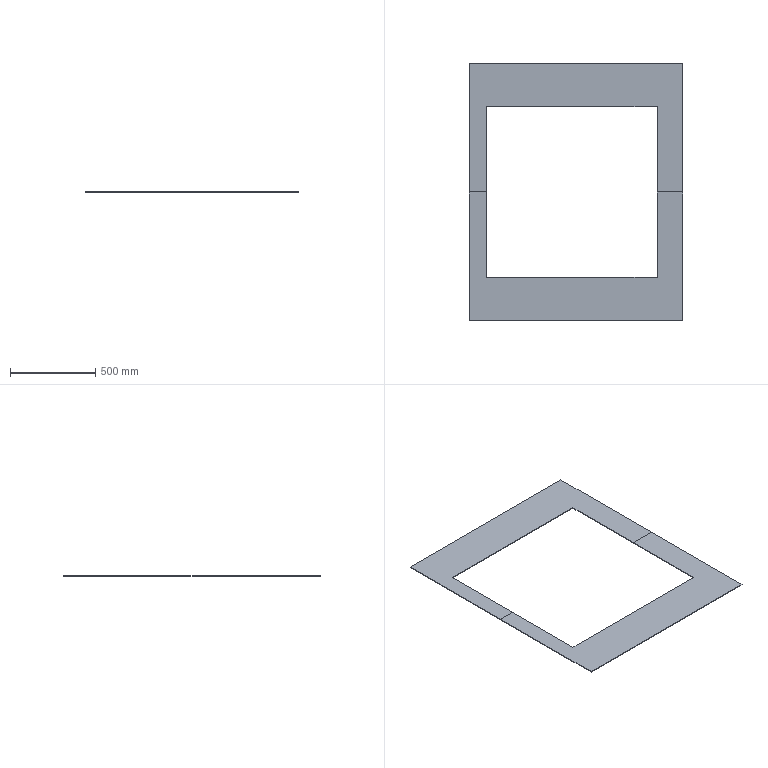Part | STEP file | 电柜通道花纹Plate 2 | 2 solids | 20 faces | box 1250 x 1500 x 4 mm | volume 3500000 mm3 | plane 20
STEP:
#1=CARTESIAN_POINT('',(0.,0.,0.));
#2=DIRECTION('',(0.,0.,1.));
#3=DIRECTION('',(1.,0.,0.));
#4=AXIS2_PLACEMENT_3D('',#1,#2,#3);
#5=CARTESIAN_POINT('',(-128.268,0.,4.));
#6=VERTEX_POINT('',#5);
#7=CARTESIAN_POINT('',(-128.268,0.,0.));
#8=VERTEX_POINT('',#7);
#9=CARTESIAN_POINT('',(-128.268,0.,0.));
#10=DIRECTION('',(0.,0.,-1.));
#11=VECTOR('',#10,1.);
#12=LINE('',#9,#11);
#13=CARTESIAN_POINT('',(-1228.268,0.,-0.01));
#14=DIRECTION('',(0.,-1.,0.));
#15=DIRECTION('',(1.,0.,0.));
#16=AXIS2_PLACEMENT_3D('',#13,#14,#15);
#17=PLANE('',#16);
#18=CARTESIAN_POINT('',(1100.,0.01));
#19=DIRECTION('',(0.,-1.));
#20=VECTOR('',#19,1.);
#21=LINE('',#18,#20);
#22=(GEOMETRIC_REPRESENTATION_CONTEXT(2)PARAMETRIC_REPRESENTATION_CONTEXT()REPRESENTATION_CONTEXT('',''));
#23=DEFINITIONAL_REPRESENTATION('',(#21),#22);
#24=PCURVE('',#17,#23);
#25=CARTESIAN_POINT('',(-128.268,-500.,0.));
#26=DIRECTION('',(1.,0.,0.));
#27=DIRECTION('',(0.,0.,-1.));
#28=AXIS2_PLACEMENT_3D('',#25,#26,#27);
#29=PLANE('',#28);
#30=CARTESIAN_POINT('',(0.,500.));
#31=DIRECTION('',(1.,0.));
#32=VECTOR('',#31,1.);
#33=LINE('',#30,#32);
#34=(GEOMETRIC_REPRESENTATION_CONTEXT(2)PARAMETRIC_REPRESENTATION_CONTEXT()REPRESENTATION_CONTEXT('',''));
#35=DEFINITIONAL_REPRESENTATION('',(#33),#34);
#36=PCURVE('',#29,#35);
#37=SURFACE_CURVE('',#12,(#24,#36),.PCURVE_S1.);
#38=EDGE_CURVE('',#6,#8,#37,.T.);
#39=ORIENTED_EDGE('',*,*,#38,.F.);
#40=CARTESIAN_POINT('',(21.732,0.,4.));
#41=VERTEX_POINT('',#40);
#42=CARTESIAN_POINT('',(0.,0.,4.));
#43=DIRECTION('',(1.,0.,0.));
#44=VECTOR('',#43,1.);
#45=LINE('',#42,#44);
#46=CARTESIAN_POINT('',(1228.268,4.01));
#47=DIRECTION('',(1.,0.));
#48=VECTOR('',#47,1.);
#49=LINE('',#46,#48);
#50=(GEOMETRIC_REPRESENTATION_CONTEXT(2)PARAMETRIC_REPRESENTATION_CONTEXT()REPRESENTATION_CONTEXT('',''));
#51=DEFINITIONAL_REPRESENTATION('',(#49),#50);
#52=PCURVE('',#17,#51);
#53=CARTESIAN_POINT('',(0.,0.,4.));
#54=DIRECTION('',(0.,0.,1.));
#55=DIRECTION('',(1.,0.,0.));
#56=AXIS2_PLACEMENT_3D('',#53,#54,#55);
#57=PLANE('',#56);
#58=CARTESIAN_POINT('',(0.,0.));
#59=DIRECTION('',(1.,0.));
#60=VECTOR('',#59,1.);
#61=LINE('',#58,#60);
#62=(GEOMETRIC_REPRESENTATION_CONTEXT(2)PARAMETRIC_REPRESENTATION_CONTEXT()REPRESENTATION_CONTEXT('',''));
#63=DEFINITIONAL_REPRESENTATION('',(#61),#62);
#64=PCURVE('',#57,#63);
#65=SURFACE_CURVE('',#45,(#52,#64),.PCURVE_S1.);
#66=EDGE_CURVE('',#6,#41,#65,.T.);
#67=ORIENTED_EDGE('',*,*,#66,.T.);
#68=CARTESIAN_POINT('',(21.732,0.,0.));
#69=VERTEX_POINT('',#68);
#70=CARTESIAN_POINT('',(21.732,0.,4.));
#71=DIRECTION('',(0.,0.,1.));
#72=VECTOR('',#71,1.);
#73=LINE('',#70,#72);
#74=CARTESIAN_POINT('',(1250.,4.01));
#75=DIRECTION('',(0.,1.));
#76=VECTOR('',#75,1.);
#77=LINE('',#74,#76);
#78=(GEOMETRIC_REPRESENTATION_CONTEXT(2)PARAMETRIC_REPRESENTATION_CONTEXT()REPRESENTATION_CONTEXT('',''));
#79=DEFINITIONAL_REPRESENTATION('',(#77),#78);
#80=PCURVE('',#17,#79);
#81=CARTESIAN_POINT('',(21.732,750.,4.));
#82=DIRECTION('',(-1.,0.,0.));
#83=DIRECTION('',(0.,-1.,0.));
#84=AXIS2_PLACEMENT_3D('',#81,#82,#83);
#85=PLANE('',#84);
#86=CARTESIAN_POINT('',(750.,0.));
#87=DIRECTION('',(0.,1.));
#88=VECTOR('',#87,1.);
#89=LINE('',#86,#88);
#90=(GEOMETRIC_REPRESENTATION_CONTEXT(2)PARAMETRIC_REPRESENTATION_CONTEXT()REPRESENTATION_CONTEXT('',''));
#91=DEFINITIONAL_REPRESENTATION('',(#89),#90);
#92=PCURVE('',#85,#91);
#93=SURFACE_CURVE('',#73,(#80,#92),.PCURVE_S1.);
#94=EDGE_CURVE('',#69,#41,#93,.T.);
#95=ORIENTED_EDGE('',*,*,#94,.F.);
#96=CARTESIAN_POINT('',(0.,0.,0.));
#97=DIRECTION('',(1.,0.,0.));
#98=VECTOR('',#97,1.);
#99=LINE('',#96,#98);
#100=CARTESIAN_POINT('',(1228.268,0.01));
#101=DIRECTION('',(1.,0.));
#102=VECTOR('',#101,1.);
#103=LINE('',#100,#102);
#104=(GEOMETRIC_REPRESENTATION_CONTEXT(2)PARAMETRIC_REPRESENTATION_CONTEXT()REPRESENTATION_CONTEXT('',''));
#105=DEFINITIONAL_REPRESENTATION('',(#103),#104);
#106=PCURVE('',#17,#105);
#107=CARTESIAN_POINT('',(0.,0.,0.));
#108=DIRECTION('',(0.,0.,1.));
#109=DIRECTION('',(1.,0.,0.));
#110=AXIS2_PLACEMENT_3D('',#107,#108,#109);
#111=PLANE('',#110);
#112=CARTESIAN_POINT('',(0.,0.));
#113=DIRECTION('',(1.,0.));
#114=VECTOR('',#113,1.);
#115=LINE('',#112,#114);
#116=(GEOMETRIC_REPRESENTATION_CONTEXT(2)PARAMETRIC_REPRESENTATION_CONTEXT()REPRESENTATION_CONTEXT('',''));
#117=DEFINITIONAL_REPRESENTATION('',(#115),#116);
#118=PCURVE('',#111,#117);
#119=SURFACE_CURVE('',#99,(#106,#118),.PCURVE_S1.);
#120=EDGE_CURVE('',#8,#69,#119,.T.);
#121=ORIENTED_EDGE('',*,*,#120,.F.);
#122=EDGE_LOOP('',(#39,#67,#95,#121));
#123=FACE_BOUND('',#122,.T.);
#124=ADVANCED_FACE('',(#123),#17,.F.);
#125=CARTESIAN_POINT('',(-1228.268,0.,4.));
#126=VERTEX_POINT('',#125);
#127=CARTESIAN_POINT('',(-1228.268,0.,0.));
#128=VERTEX_POINT('',#127);
#129=CARTESIAN_POINT('',(-1228.268,0.,4.));
#130=DIRECTION('',(0.,0.,-1.));
#131=VECTOR('',#130,1.);
#132=LINE('',#129,#131);
#133=CARTESIAN_POINT('',(-1228.268,0.,-0.01));
#134=DIRECTION('',(0.,-1.,0.));
#135=DIRECTION('',(1.,0.,0.));
#136=AXIS2_PLACEMENT_3D('',#133,#134,#135);
#137=PLANE('',#136);
#138=CARTESIAN_POINT('',(0.,4.01));
#139=DIRECTION('',(0.,-1.));
#140=VECTOR('',#139,1.);
#141=LINE('',#138,#140);
#142=(GEOMETRIC_REPRESENTATION_CONTEXT(2)PARAMETRIC_REPRESENTATION_CONTEXT()REPRESENTATION_CONTEXT('',''));
#143=DEFINITIONAL_REPRESENTATION('',(#141),#142);
#144=PCURVE('',#137,#143);
#145=CARTESIAN_POINT('',(-1228.268,750.,4.));
#146=DIRECTION('',(1.,0.,0.));
#147=DIRECTION('',(0.,1.,0.));
#148=AXIS2_PLACEMENT_3D('',#145,#146,#147);
#149=PLANE('',#148);
#150=CARTESIAN_POINT('',(-750.,0.));
#151=DIRECTION('',(0.,-1.));
#152=VECTOR('',#151,1.);
#153=LINE('',#150,#152);
#154=(GEOMETRIC_REPRESENTATION_CONTEXT(2)PARAMETRIC_REPRESENTATION_CONTEXT()REPRESENTATION_CONTEXT('',''));
#155=DEFINITIONAL_REPRESENTATION('',(#153),#154);
#156=PCURVE('',#149,#155);
#157=SURFACE_CURVE('',#132,(#144,#156),.PCURVE_S1.);
#158=EDGE_CURVE('',#126,#128,#157,.T.);
#159=ORIENTED_EDGE('',*,*,#158,.F.);
#160=CARTESIAN_POINT('',(-1128.268,0.,4.));
#161=VERTEX_POINT('',#160);
#162=CARTESIAN_POINT('',(0.,0.,4.));
#163=DIRECTION('',(1.,0.,0.));
#164=VECTOR('',#163,1.);
#165=LINE('',#162,#164);
#166=CARTESIAN_POINT('',(1228.268,4.01));
#167=DIRECTION('',(1.,0.));
#168=VECTOR('',#167,1.);
#169=LINE('',#166,#168);
#170=(GEOMETRIC_REPRESENTATION_CONTEXT(2)PARAMETRIC_REPRESENTATION_CONTEXT()REPRESENTATION_CONTEXT('',''));
#171=DEFINITIONAL_REPRESENTATION('',(#169),#170);
#172=PCURVE('',#137,#171);
#173=CARTESIAN_POINT('',(0.,0.));
#174=DIRECTION('',(1.,0.));
#175=VECTOR('',#174,1.);
#176=LINE('',#173,#175);
#177=(GEOMETRIC_REPRESENTATION_CONTEXT(2)PARAMETRIC_REPRESENTATION_CONTEXT()REPRESENTATION_CONTEXT('',''));
#178=DEFINITIONAL_REPRESENTATION('',(#176),#177);
#179=PCURVE('',#57,#178);
#180=SURFACE_CURVE('',#165,(#172,#179),.PCURVE_S1.);
#181=EDGE_CURVE('',#126,#161,#180,.T.);
#182=ORIENTED_EDGE('',*,*,#181,.T.);
#183=CARTESIAN_POINT('',(-1128.268,0.,0.));
#184=VERTEX_POINT('',#183);
#185=CARTESIAN_POINT('',(-1128.268,0.,0.));
#186=DIRECTION('',(0.,0.,1.));
#187=VECTOR('',#186,1.);
#188=LINE('',#185,#187);
#189=CARTESIAN_POINT('',(100.,0.01));
#190=DIRECTION('',(0.,1.));
#191=VECTOR('',#190,1.);
#192=LINE('',#189,#191);
#193=(GEOMETRIC_REPRESENTATION_CONTEXT(2)PARAMETRIC_REPRESENTATION_CONTEXT()REPRESENTATION_CONTEXT('',''));
#194=DEFINITIONAL_REPRESENTATION('',(#192),#193);
#195=PCURVE('',#137,#194);
#196=CARTESIAN_POINT('',(-1128.268,-500.,0.));
#197=DIRECTION('',(-1.,0.,0.));
#198=DIRECTION('',(0.,0.,1.));
#199=AXIS2_PLACEMENT_3D('',#196,#197,#198);
#200=PLANE('',#199);
#201=CARTESIAN_POINT('',(0.,500.));
#202=DIRECTION('',(1.,0.));
#203=VECTOR('',#202,1.);
#204=LINE('',#201,#203);
#205=(GEOMETRIC_REPRESENTATION_CONTEXT(2)PARAMETRIC_REPRESENTATION_CONTEXT()REPRESENTATION_CONTEXT('',''));
#206=DEFINITIONAL_REPRESENTATION('',(#204),#205);
#207=PCURVE('',#200,#206);
#208=SURFACE_CURVE('',#188,(#195,#207),.PCURVE_S1.);
#209=EDGE_CURVE('',#184,#161,#208,.T.);
#210=ORIENTED_EDGE('',*,*,#209,.F.);
#211=CARTESIAN_POINT('',(0.,0.,0.));
#212=DIRECTION('',(1.,0.,0.));
#213=VECTOR('',#212,1.);
#214=LINE('',#211,#213);
#215=CARTESIAN_POINT('',(1228.268,0.01));
#216=DIRECTION('',(1.,0.));
#217=VECTOR('',#216,1.);
#218=LINE('',#215,#217);
#219=(GEOMETRIC_REPRESENTATION_CONTEXT(2)PARAMETRIC_REPRESENTATION_CONTEXT()REPRESENTATION_CONTEXT('',''));
#220=DEFINITIONAL_REPRESENTATION('',(#218),#219);
#221=PCURVE('',#137,#220);
#222=CARTESIAN_POINT('',(0.,0.));
#223=DIRECTION('',(1.,0.));
#224=VECTOR('',#223,1.);
#225=LINE('',#222,#224);
#226=(GEOMETRIC_REPRESENTATION_CONTEXT(2)PARAMETRIC_REPRESENTATION_CONTEXT()REPRESENTATION_CONTEXT('',''));
#227=DEFINITIONAL_REPRESENTATION('',(#225),#226);
#228=PCURVE('',#111,#227);
#229=SURFACE_CURVE('',#214,(#221,#228),.PCURVE_S1.);
#230=EDGE_CURVE('',#128,#184,#229,.T.);
#231=ORIENTED_EDGE('',*,*,#230,.F.);
#232=EDGE_LOOP('',(#159,#182,#210,#231));
#233=FACE_BOUND('',#232,.T.);
#234=ADVANCED_FACE('',(#233),#137,.F.);
#235=CARTESIAN_POINT('',(-128.268,-500.,4.));
#236=VERTEX_POINT('',#235);
#237=CARTESIAN_POINT('',(-128.268,-500.,4.));
#238=DIRECTION('',(0.,1.,0.));
#239=VECTOR('',#238,1.);
#240=LINE('',#237,#239);
#241=CARTESIAN_POINT('',(-4.,0.));
#242=DIRECTION('',(0.,1.));
#243=VECTOR('',#242,1.);
#244=LINE('',#241,#243);
#245=(GEOMETRIC_REPRESENTATION_CONTEXT(2)PARAMETRIC_REPRESENTATION_CONTEXT()REPRESENTATION_CONTEXT('',''));
#246=DEFINITIONAL_REPRESENTATION('',(#244),#245);
#247=PCURVE('',#29,#246);
#248=CARTESIAN_POINT('',(-128.268,-500.));
#249=DIRECTION('',(0.,1.));
#250=VECTOR('',#249,1.);
#251=LINE('',#248,#250);
#252=(GEOMETRIC_REPRESENTATION_CONTEXT(2)PARAMETRIC_REPRESENTATION_CONTEXT()REPRESENTATION_CONTEXT('',''));
#253=DEFINITIONAL_REPRESENTATION('',(#251),#252);
#254=PCURVE('',#57,#253);
#255=SURFACE_CURVE('',#240,(#247,#254),.PCURVE_S1.);
#256=EDGE_CURVE('',#236,#6,#255,.T.);
#257=ORIENTED_EDGE('',*,*,#256,.T.);
#258=ORIENTED_EDGE('',*,*,#38,.T.);
#259=CARTESIAN_POINT('',(-128.268,-500.,0.));
#260=VERTEX_POINT('',#259);
#261=CARTESIAN_POINT('',(-128.268,-500.,0.));
#262=DIRECTION('',(0.,1.,0.));
#263=VECTOR('',#262,1.);
#264=LINE('',#261,#263);
#265=CARTESIAN_POINT('',(0.,0.));
#266=DIRECTION('',(0.,1.));
#267=VECTOR('',#266,1.);
#268=LINE('',#265,#267);
#269=(GEOMETRIC_REPRESENTATION_CONTEXT(2)PARAMETRIC_REPRESENTATION_CONTEXT()REPRESENTATION_CONTEXT('',''));
#270=DEFINITIONAL_REPRESENTATION('',(#268),#269);
#271=PCURVE('',#29,#270);
#272=CARTESIAN_POINT('',(-128.268,-500.));
#273=DIRECTION('',(0.,1.));
#274=VECTOR('',#273,1.);
#275=LINE('',#272,#274);
#276=(GEOMETRIC_REPRESENTATION_CONTEXT(2)PARAMETRIC_REPRESENTATION_CONTEXT()REPRESENTATION_CONTEXT('',''));
#277=DEFINITIONAL_REPRESENTATION('',(#275),#276);
#278=PCURVE('',#111,#277);
#279=SURFACE_CURVE('',#264,(#271,#278),.PCURVE_S1.);
#280=EDGE_CURVE('',#260,#8,#279,.T.);
#281=ORIENTED_EDGE('',*,*,#280,.F.);
#282=CARTESIAN_POINT('',(-128.268,-500.,0.));
#283=DIRECTION('',(0.,0.,1.));
#284=VECTOR('',#283,1.);
#285=LINE('',#282,#284);
#286=CARTESIAN_POINT('',(0.,0.));
#287=DIRECTION('',(-1.,0.));
#288=VECTOR('',#287,1.);
#289=LINE('',#286,#288);
#290=(GEOMETRIC_REPRESENTATION_CONTEXT(2)PARAMETRIC_REPRESENTATION_CONTEXT()REPRESENTATION_CONTEXT('',''));
#291=DEFINITIONAL_REPRESENTATION('',(#289),#290);
#292=PCURVE('',#29,#291);
#293=CARTESIAN_POINT('',(-1128.268,-500.,0.));
#294=DIRECTION('',(0.,-1.,0.));
#295=DIRECTION('',(0.,0.,-1.));
#296=AXIS2_PLACEMENT_3D('',#293,#294,#295);
#297=PLANE('',#296);
#298=CARTESIAN_POINT('',(0.,1000.));
#299=DIRECTION('',(-1.,0.));
#300=VECTOR('',#299,1.);
#301=LINE('',#298,#300);
#302=(GEOMETRIC_REPRESENTATION_CONTEXT(2)PARAMETRIC_REPRESENTATION_CONTEXT()REPRESENTATION_CONTEXT('',''));
#303=DEFINITIONAL_REPRESENTATION('',(#301),#302);
#304=PCURVE('',#297,#303);
#305=SURFACE_CURVE('',#285,(#292,#304),.PCURVE_S1.);
#306=EDGE_CURVE('',#260,#236,#305,.T.);
#307=ORIENTED_EDGE('',*,*,#306,.T.);
#308=EDGE_LOOP('',(#257,#258,#281,#307));
#309=FACE_BOUND('',#308,.T.);
#310=ADVANCED_FACE('',(#309),#29,.F.);
#311=CARTESIAN_POINT('',(-1128.268,-500.,0.));
#312=VERTEX_POINT('',#311);
#313=CARTESIAN_POINT('',(-1128.268,-500.,0.));
#314=DIRECTION('',(0.,-1.,0.));
#315=VECTOR('',#314,1.);
#316=LINE('',#313,#315);
#317=CARTESIAN_POINT('',(0.,0.));
#318=DIRECTION('',(0.,-1.));
#319=VECTOR('',#318,1.);
#320=LINE('',#317,#319);
#321=(GEOMETRIC_REPRESENTATION_CONTEXT(2)PARAMETRIC_REPRESENTATION_CONTEXT()REPRESENTATION_CONTEXT('',''));
#322=DEFINITIONAL_REPRESENTATION('',(#320),#321);
#323=PCURVE('',#200,#322);
#324=CARTESIAN_POINT('',(-1128.268,-500.));
#325=DIRECTION('',(0.,-1.));
#326=VECTOR('',#325,1.);
#327=LINE('',#324,#326);
#328=(GEOMETRIC_REPRESENTATION_CONTEXT(2)PARAMETRIC_REPRESENTATION_CONTEXT()REPRESENTATION_CONTEXT('',''));
#329=DEFINITIONAL_REPRESENTATION('',(#327),#328);
#330=PCURVE('',#111,#329);
#331=SURFACE_CURVE('',#316,(#323,#330),.PCURVE_S1.);
#332=EDGE_CURVE('',#184,#312,#331,.T.);
#333=ORIENTED_EDGE('',*,*,#332,.F.);
#334=ORIENTED_EDGE('',*,*,#209,.T.);
#335=CARTESIAN_POINT('',(-1128.268,-500.,4.));
#336=VERTEX_POINT('',#335);
#337=CARTESIAN_POINT('',(-1128.268,-500.,4.));
#338=DIRECTION('',(0.,-1.,0.));
#339=VECTOR('',#338,1.);
#340=LINE('',#337,#339);
#341=CARTESIAN_POINT('',(4.,0.));
#342=DIRECTION('',(0.,-1.));
#343=VECTOR('',#342,1.);
#344=LINE('',#341,#343);
#345=(GEOMETRIC_REPRESENTATION_CONTEXT(2)PARAMETRIC_REPRESENTATION_CONTEXT()REPRESENTATION_CONTEXT('',''));
#346=DEFINITIONAL_REPRESENTATION('',(#344),#345);
#347=PCURVE('',#200,#346);
#348=CARTESIAN_POINT('',(-1128.268,-500.));
#349=DIRECTION('',(0.,-1.));
#350=VECTOR('',#349,1.);
#351=LINE('',#348,#350);
#352=(GEOMETRIC_REPRESENTATION_CONTEXT(2)PARAMETRIC_REPRESENTATION_CONTEXT()REPRESENTATION_CONTEXT('',''));
#353=DEFINITIONAL_REPRESENTATION('',(#351),#352);
#354=PCURVE('',#57,#353);
#355=SURFACE_CURVE('',#340,(#347,#354),.PCURVE_S1.);
#356=EDGE_CURVE('',#161,#336,#355,.T.);
#357=ORIENTED_EDGE('',*,*,#356,.T.);
#358=CARTESIAN_POINT('',(-1128.268,-500.,0.));
#359=DIRECTION('',(0.,0.,1.));
#360=VECTOR('',#359,1.);
#361=LINE('',#358,#360);
#362=CARTESIAN_POINT('',(0.,0.));
#363=DIRECTION('',(1.,0.));
#364=VECTOR('',#363,1.);
#365=LINE('',#362,#364);
#366=(GEOMETRIC_REPRESENTATION_CONTEXT(2)PARAMETRIC_REPRESENTATION_CONTEXT()REPRESENTATION_CONTEXT('',''));
#367=DEFINITIONAL_REPRESENTATION('',(#365),#366);
#368=PCURVE('',#200,#367);
#369=CARTESIAN_POINT('',(0.,0.));
#370=DIRECTION('',(-1.,0.));
#371=VECTOR('',#370,1.);
#372=LINE('',#369,#371);
#373=(GEOMETRIC_REPRESENTATION_CONTEXT(2)PARAMETRIC_REPRESENTATION_CONTEXT()REPRESENTATION_CONTEXT('',''));
#374=DEFINITIONAL_REPRESENTATION('',(#372),#373);
#375=PCURVE('',#297,#374);
#376=SURFACE_CURVE('',#361,(#368,#375),.PCURVE_S1.);
#377=EDGE_CURVE('',#312,#336,#376,.T.);
#378=ORIENTED_EDGE('',*,*,#377,.F.);
#379=EDGE_LOOP('',(#333,#334,#357,#378));
#380=FACE_BOUND('',#379,.T.);
#381=ADVANCED_FACE('',(#380),#200,.F.);
#382=CARTESIAN_POINT('',(-1228.268,-750.,0.));
#383=VERTEX_POINT('',#382);
#384=CARTESIAN_POINT('',(-1228.268,750.,0.));
#385=DIRECTION('',(0.,-1.,0.));
#386=VECTOR('',#385,1.);
#387=LINE('',#384,#386);
#388=CARTESIAN_POINT('',(-1228.268,750.));
#389=DIRECTION('',(0.,-1.));
#390=VECTOR('',#389,1.);
#391=LINE('',#388,#390);
#392=(GEOMETRIC_REPRESENTATION_CONTEXT(2)PARAMETRIC_REPRESENTATION_CONTEXT()REPRESENTATION_CONTEXT('',''));
#393=DEFINITIONAL_REPRESENTATION('',(#391),#392);
#394=PCURVE('',#111,#393);
#395=CARTESIAN_POINT('',(0.,-4.));
#396=DIRECTION('',(-1.,0.));
#397=VECTOR('',#396,1.);
#398=LINE('',#395,#397);
#399=(GEOMETRIC_REPRESENTATION_CONTEXT(2)PARAMETRIC_REPRESENTATION_CONTEXT()REPRESENTATION_CONTEXT('',''));
#400=DEFINITIONAL_REPRESENTATION('',(#398),#399);
#401=PCURVE('',#149,#400);
#402=SURFACE_CURVE('',#387,(#394,#401),.PCURVE_S1.);
#403=EDGE_CURVE('',#128,#383,#402,.T.);
#404=ORIENTED_EDGE('',*,*,#403,.F.);
#405=ORIENTED_EDGE('',*,*,#230,.T.);
#406=ORIENTED_EDGE('',*,*,#332,.T.);
#407=CARTESIAN_POINT('',(-1128.268,-500.,0.));
#408=DIRECTION('',(1.,0.,0.));
#409=VECTOR('',#408,1.);
#410=LINE('',#407,#409);
#411=CARTESIAN_POINT('',(-1128.268,-500.));
#412=DIRECTION('',(1.,0.));
#413=VECTOR('',#412,1.);
#414=LINE('',#411,#413);
#415=(GEOMETRIC_REPRESENTATION_CONTEXT(2)PARAMETRIC_REPRESENTATION_CONTEXT()REPRESENTATION_CONTEXT('',''));
#416=DEFINITIONAL_REPRESENTATION('',(#414),#415);
#417=PCURVE('',#111,#416);
#418=CARTESIAN_POINT('',(0.,0.));
#419=DIRECTION('',(0.,1.));
#420=VECTOR('',#419,1.);
#421=LINE('',#418,#420);
#422=(GEOMETRIC_REPRESENTATION_CONTEXT(2)PARAMETRIC_REPRESENTATION_CONTEXT()REPRESENTATION_CONTEXT('',''));
#423=DEFINITIONAL_REPRESENTATION('',(#421),#422);
#424=PCURVE('',#297,#423);
#425=SURFACE_CURVE('',#410,(#417,#424),.PCURVE_S1.);
#426=EDGE_CURVE('',#312,#260,#425,.T.);
#427=ORIENTED_EDGE('',*,*,#426,.T.);
#428=ORIENTED_EDGE('',*,*,#280,.T.);
#429=ORIENTED_EDGE('',*,*,#120,.T.);
#430=CARTESIAN_POINT('',(21.732,-750.,0.));
#431=VERTEX_POINT('',#430);
#432=CARTESIAN_POINT('',(21.732,750.,0.));
#433=DIRECTION('',(0.,1.,0.));
#434=VECTOR('',#433,1.);
#435=LINE('',#432,#434);
#436=CARTESIAN_POINT('',(21.732,750.));
#437=DIRECTION('',(0.,1.));
#438=VECTOR('',#437,1.);
#439=LINE('',#436,#438);
#440=(GEOMETRIC_REPRESENTATION_CONTEXT(2)PARAMETRIC_REPRESENTATION_CONTEXT()REPRESENTATION_CONTEXT('',''));
#441=DEFINITIONAL_REPRESENTATION('',(#439),#440);
#442=PCURVE('',#111,#441);
#443=CARTESIAN_POINT('',(0.,-4.));
#444=DIRECTION('',(-1.,0.));
#445=VECTOR('',#444,1.);
#446=LINE('',#443,#445);
#447=(GEOMETRIC_REPRESENTATION_CONTEXT(2)PARAMETRIC_REPRESENTATION_CONTEXT()REPRESENTATION_CONTEXT('',''));
#448=DEFINITIONAL_REPRESENTATION('',(#446),#447);
#449=PCURVE('',#85,#448);
#450=SURFACE_CURVE('',#435,(#442,#449),.PCURVE_S1.);
#451=EDGE_CURVE('',#431,#69,#450,.T.);
#452=ORIENTED_EDGE('',*,*,#451,.F.);
#453=CARTESIAN_POINT('',(-1228.268,-750.,0.));
#454=DIRECTION('',(1.,0.,0.));
#455=VECTOR('',#454,1.);
#456=LINE('',#453,#455);
#457=CARTESIAN_POINT('',(-1228.268,-750.));
#458=DIRECTION('',(1.,0.));
#459=VECTOR('',#458,1.);
#460=LINE('',#457,#459);
#461=(GEOMETRIC_REPRESENTATION_CONTEXT(2)PARAMETRIC_REPRESENTATION_CONTEXT()REPRESENTATION_CONTEXT('',''));
#462=DEFINITIONAL_REPRESENTATION('',(#460),#461);
#463=PCURVE('',#111,#462);
#464=CARTESIAN_POINT('',(-1228.268,-750.,4.));
#465=DIRECTION('',(0.,1.,0.));
#466=DIRECTION('',(0.,0.,1.));
#467=AXIS2_PLACEMENT_3D('',#464,#465,#466);
#468=PLANE('',#467);
#469=CARTESIAN_POINT('',(-4.,0.));
#470=DIRECTION('',(0.,1.));
#471=VECTOR('',#470,1.);
#472=LINE('',#469,#471);
#473=(GEOMETRIC_REPRESENTATION_CONTEXT(2)PARAMETRIC_REPRESENTATION_CONTEXT()REPRESENTATION_CONTEXT('',''));
#474=DEFINITIONAL_REPRESENTATION('',(#472),#473);
#475=PCURVE('',#468,#474);
#476=SURFACE_CURVE('',#456,(#463,#475),.PCURVE_S1.);
#477=EDGE_CURVE('',#383,#431,#476,.T.);
#478=ORIENTED_EDGE('',*,*,#477,.F.);
#479=EDGE_LOOP('',(#404,#405,#406,#427,#428,#429,#452,#478));
#480=FACE_BOUND('',#479,.T.);
#481=ADVANCED_FACE('',(#480),#111,.F.);
#482=ORIENTED_EDGE('',*,*,#181,.F.);
#483=CARTESIAN_POINT('',(-1228.268,-750.,4.));
#484=VERTEX_POINT('',#483);
#485=CARTESIAN_POINT('',(-1228.268,750.,4.));
#486=DIRECTION('',(0.,-1.,0.));
#487=VECTOR('',#486,1.);
#488=LINE('',#485,#487);
#489=CARTESIAN_POINT('',(-1228.268,750.));
#490=DIRECTION('',(0.,-1.));
#491=VECTOR('',#490,1.);
#492=LINE('',#489,#491);
#493=(GEOMETRIC_REPRESENTATION_CONTEXT(2)PARAMETRIC_REPRESENTATION_CONTEXT()REPRESENTATION_CONTEXT('',''));
#494=DEFINITIONAL_REPRESENTATION('',(#492),#493);
#495=PCURVE('',#57,#494);
#496=CARTESIAN_POINT('',(0.,0.));
#497=DIRECTION('',(-1.,0.));
#498=VECTOR('',#497,1.);
#499=LINE('',#496,#498);
#500=(GEOMETRIC_REPRESENTATION_CONTEXT(2)PARAMETRIC_REPRESENTATION_CONTEXT()REPRESENTATION_CONTEXT('',''));
#501=DEFINITIONAL_REPRESENTATION('',(#499),#500);
#502=PCURVE('',#149,#501);
#503=SURFACE_CURVE('',#488,(#495,#502),.PCURVE_S1.);
#504=EDGE_CURVE('',#126,#484,#503,.T.);
#505=ORIENTED_EDGE('',*,*,#504,.T.);
#506=CARTESIAN_POINT('',(21.732,-750.,4.));
#507=VERTEX_POINT('',#506);
#508=CARTESIAN_POINT('',(-1228.268,-750.,4.));
#509=DIRECTION('',(1.,0.,0.));
#510=VECTOR('',#509,1.);
#511=LINE('',#508,#510);
#512=CARTESIAN_POINT('',(-1228.268,-750.));
#513=DIRECTION('',(1.,0.));
#514=VECTOR('',#513,1.);
#515=LINE('',#512,#514);
#516=(GEOMETRIC_REPRESENTATION_CONTEXT(2)PARAMETRIC_REPRESENTATION_CONTEXT()REPRESENTATION_CONTEXT('',''));
#517=DEFINITIONAL_REPRESENTATION('',(#515),#516);
#518=PCURVE('',#57,#517);
#519=CARTESIAN_POINT('',(0.,0.));
#520=DIRECTION('',(0.,1.));
#521=VECTOR('',#520,1.);
#522=LINE('',#519,#521);
#523=(GEOMETRIC_REPRESENTATION_CONTEXT(2)PARAMETRIC_REPRESENTATION_CONTEXT()REPRESENTATION_CONTEXT('',''));
#524=DEFINITIONAL_REPRESENTATION('',(#522),#523);
#525=PCURVE('',#468,#524);
#526=SURFACE_CURVE('',#511,(#518,#525),.PCURVE_S1.);
#527=EDGE_CURVE('',#484,#507,#526,.T.);
#528=ORIENTED_EDGE('',*,*,#527,.T.);
#529=CARTESIAN_POINT('',(21.732,750.,4.));
#530=DIRECTION('',(0.,1.,0.));
#531=VECTOR('',#530,1.);
#532=LINE('',#529,#531);
#533=CARTESIAN_POINT('',(21.732,750.));
#534=DIRECTION('',(0.,1.));
#535=VECTOR('',#534,1.);
#536=LINE('',#533,#535);
#537=(GEOMETRIC_REPRESENTATION_CONTEXT(2)PARAMETRIC_REPRESENTATION_CONTEXT()REPRESENTATION_CONTEXT('',''));
#538=DEFINITIONAL_REPRESENTATION('',(#536),#537);
#539=PCURVE('',#57,#538);
#540=CARTESIAN_POINT('',(0.,0.));
#541=DIRECTION('',(-1.,0.));
#542=VECTOR('',#541,1.);
#543=LINE('',#540,#542);
#544=(GEOMETRIC_REPRESENTATION_CONTEXT(2)PARAMETRIC_REPRESENTATION_CONTEXT()REPRESENTATION_CONTEXT('',''));
#545=DEFINITIONAL_REPRESENTATION('',(#543),#544);
#546=PCURVE('',#85,#545);
#547=SURFACE_CURVE('',#532,(#539,#546),.PCURVE_S1.);
#548=EDGE_CURVE('',#507,#41,#547,.T.);
#549=ORIENTED_EDGE('',*,*,#548,.T.);
#550=ORIENTED_EDGE('',*,*,#66,.F.);
#551=ORIENTED_EDGE('',*,*,#256,.F.);
#552=CARTESIAN_POINT('',(-1128.268,-500.,4.));
#553=DIRECTION('',(1.,0.,0.));
#554=VECTOR('',#553,1.);
#555=LINE('',#552,#554);
#556=CARTESIAN_POINT('',(-1128.268,-500.));
#557=DIRECTION('',(1.,0.));
#558=VECTOR('',#557,1.);
#559=LINE('',#556,#558);
#560=(GEOMETRIC_REPRESENTATION_CONTEXT(2)PARAMETRIC_REPRESENTATION_CONTEXT()REPRESENTATION_CONTEXT('',''));
#561=DEFINITIONAL_REPRESENTATION('',(#559),#560);
#562=PCURVE('',#57,#561);
#563=CARTESIAN_POINT('',(-4.,0.));
#564=DIRECTION('',(0.,1.));
#565=VECTOR('',#564,1.);
#566=LINE('',#563,#565);
#567=(GEOMETRIC_REPRESENTATION_CONTEXT(2)PARAMETRIC_REPRESENTATION_CONTEXT()REPRESENTATION_CONTEXT('',''));
#568=DEFINITIONAL_REPRESENTATION('',(#566),#567);
#569=PCURVE('',#297,#568);
#570=SURFACE_CURVE('',#555,(#562,#569),.PCURVE_S1.);
#571=EDGE_CURVE('',#336,#236,#570,.T.);
#572=ORIENTED_EDGE('',*,*,#571,.F.);
#573=ORIENTED_EDGE('',*,*,#356,.F.);
#574=EDGE_LOOP('',(#482,#505,#528,#549,#550,#551,#572,#573));
#575=FACE_BOUND('',#574,.T.);
#576=ADVANCED_FACE('',(#575),#57,.T.);
#577=ORIENTED_EDGE('',*,*,#571,.T.);
#578=ORIENTED_EDGE('',*,*,#306,.F.);
#579=ORIENTED_EDGE('',*,*,#426,.F.);
#580=ORIENTED_EDGE('',*,*,#377,.T.);
#581=EDGE_LOOP('',(#577,#578,#579,#580));
#582=FACE_BOUND('',#581,.T.);
#583=ADVANCED_FACE('',(#582),#297,.F.);
#584=ORIENTED_EDGE('',*,*,#504,.F.);
#585=ORIENTED_EDGE('',*,*,#158,.T.);
#586=ORIENTED_EDGE('',*,*,#403,.T.);
#587=CARTESIAN_POINT('',(-1228.268,-750.,4.));
#588=DIRECTION('',(0.,0.,-1.));
#589=VECTOR('',#588,1.);
#590=LINE('',#587,#589);
#591=CARTESIAN_POINT('',(-1500.,0.));
#592=DIRECTION('',(0.,-1.));
#593=VECTOR('',#592,1.);
#594=LINE('',#591,#593);
#595=(GEOMETRIC_REPRESENTATION_CONTEXT(2)PARAMETRIC_REPRESENTATION_CONTEXT()REPRESENTATION_CONTEXT('',''));
#596=DEFINITIONAL_REPRESENTATION('',(#594),#595);
#597=PCURVE('',#149,#596);
#598=CARTESIAN_POINT('',(0.,0.));
#599=DIRECTION('',(-1.,0.));
#600=VECTOR('',#599,1.);
#601=LINE('',#598,#600);
#602=(GEOMETRIC_REPRESENTATION_CONTEXT(2)PARAMETRIC_REPRESENTATION_CONTEXT()REPRESENTATION_CONTEXT('',''));
#603=DEFINITIONAL_REPRESENTATION('',(#601),#602);
#604=PCURVE('',#468,#603);
#605=SURFACE_CURVE('',#590,(#597,#604),.PCURVE_S1.);
#606=EDGE_CURVE('',#484,#383,#605,.T.);
#607=ORIENTED_EDGE('',*,*,#606,.F.);
#608=EDGE_LOOP('',(#584,#585,#586,#607));
#609=FACE_BOUND('',#608,.T.);
#610=ADVANCED_FACE('',(#609),#149,.F.);
#611=ORIENTED_EDGE('',*,*,#451,.T.);
#612=ORIENTED_EDGE('',*,*,#94,.T.);
#613=ORIENTED_EDGE('',*,*,#548,.F.);
#614=CARTESIAN_POINT('',(21.732,-750.,4.));
#615=DIRECTION('',(0.,0.,-1.));
#616=VECTOR('',#615,1.);
#617=LINE('',#614,#616);
#618=CARTESIAN_POINT('',(1500.,0.));
#619=DIRECTION('',(0.,-1.));
#620=VECTOR('',#619,1.);
#621=LINE('',#618,#620);
#622=(GEOMETRIC_REPRESENTATION_CONTEXT(2)PARAMETRIC_REPRESENTATION_CONTEXT()REPRESENTATION_CONTEXT('',''));
#623=DEFINITIONAL_REPRESENTATION('',(#621),#622);
#624=PCURVE('',#85,#623);
#625=CARTESIAN_POINT('',(0.,1250.));
#626=DIRECTION('',(-1.,0.));
#627=VECTOR('',#626,1.);
#628=LINE('',#625,#627);
#629=(GEOMETRIC_REPRESENTATION_CONTEXT(2)PARAMETRIC_REPRESENTATION_CONTEXT()REPRESENTATION_CONTEXT('',''));
#630=DEFINITIONAL_REPRESENTATION('',(#628),#629);
#631=PCURVE('',#468,#630);
#632=SURFACE_CURVE('',#617,(#624,#631),.PCURVE_S1.);
#633=EDGE_CURVE('',#507,#431,#632,.T.);
#634=ORIENTED_EDGE('',*,*,#633,.T.);
#635=EDGE_LOOP('',(#611,#612,#613,#634));
#636=FACE_BOUND('',#635,.T.);
#637=ADVANCED_FACE('',(#636),#85,.F.);
#638=ORIENTED_EDGE('',*,*,#477,.T.);
#639=ORIENTED_EDGE('',*,*,#633,.F.);
#640=ORIENTED_EDGE('',*,*,#527,.F.);
#641=ORIENTED_EDGE('',*,*,#606,.T.);
#642=EDGE_LOOP('',(#638,#639,#640,#641));
#643=FACE_BOUND('',#642,.T.);
#644=ADVANCED_FACE('',(#643),#468,.F.);
#645=CLOSED_SHELL('',(#124,#234,#310,#381,#481,#576,#583,#610,#637,#644));
#646=MANIFOLD_SOLID_BREP('',#645);
#647=CARTESIAN_POINT('',(21.732,0.,0.));
#648=VERTEX_POINT('',#647);
#649=CARTESIAN_POINT('',(21.732,0.,4.));
#650=VERTEX_POINT('',#649);
#651=CARTESIAN_POINT('',(21.732,0.,4.));
#652=DIRECTION('',(0.,0.,1.));
#653=VECTOR('',#652,1.);
#654=LINE('',#651,#653);
#655=CARTESIAN_POINT('',(21.732,750.,4.));
#656=DIRECTION('',(-1.,0.,0.));
#657=DIRECTION('',(0.,-1.,0.));
#658=AXIS2_PLACEMENT_3D('',#655,#656,#657);
#659=PLANE('',#658);
#660=CARTESIAN_POINT('',(750.,0.));
#661=DIRECTION('',(0.,1.));
#662=VECTOR('',#661,1.);
#663=LINE('',#660,#662);
#664=(GEOMETRIC_REPRESENTATION_CONTEXT(2)PARAMETRIC_REPRESENTATION_CONTEXT()REPRESENTATION_CONTEXT('',''));
#665=DEFINITIONAL_REPRESENTATION('',(#663),#664);
#666=PCURVE('',#659,#665);
#667=CARTESIAN_POINT('',(-1228.268,0.,-0.01));
#668=DIRECTION('',(0.,-1.,0.));
#669=DIRECTION('',(1.,0.,0.));
#670=AXIS2_PLACEMENT_3D('',#667,#668,#669);
#671=PLANE('',#670);
#672=CARTESIAN_POINT('',(1250.,4.01));
#673=DIRECTION('',(0.,1.));
#674=VECTOR('',#673,1.);
#675=LINE('',#672,#674);
#676=(GEOMETRIC_REPRESENTATION_CONTEXT(2)PARAMETRIC_REPRESENTATION_CONTEXT()REPRESENTATION_CONTEXT('',''));
#677=DEFINITIONAL_REPRESENTATION('',(#675),#676);
#678=PCURVE('',#671,#677);
#679=SURFACE_CURVE('',#654,(#666,#678),.PCURVE_S1.);
#680=EDGE_CURVE('',#648,#650,#679,.T.);
#681=ORIENTED_EDGE('',*,*,#680,.F.);
#682=CARTESIAN_POINT('',(21.732,750.,0.));
#683=VERTEX_POINT('',#682);
#684=CARTESIAN_POINT('',(21.732,750.,0.));
#685=DIRECTION('',(0.,1.,0.));
#686=VECTOR('',#685,1.);
#687=LINE('',#684,#686);
#688=CARTESIAN_POINT('',(0.,-4.));
#689=DIRECTION('',(-1.,0.));
#690=VECTOR('',#689,1.);
#691=LINE('',#688,#690);
#692=(GEOMETRIC_REPRESENTATION_CONTEXT(2)PARAMETRIC_REPRESENTATION_CONTEXT()REPRESENTATION_CONTEXT('',''));
#693=DEFINITIONAL_REPRESENTATION('',(#691),#692);
#694=PCURVE('',#659,#693);
#695=CARTESIAN_POINT('',(0.,0.,0.));
#696=DIRECTION('',(0.,0.,1.));
#697=DIRECTION('',(1.,0.,0.));
#698=AXIS2_PLACEMENT_3D('',#695,#696,#697);
#699=PLANE('',#698);
#700=CARTESIAN_POINT('',(21.732,750.));
#701=DIRECTION('',(0.,1.));
#702=VECTOR('',#701,1.);
#703=LINE('',#700,#702);
#704=(GEOMETRIC_REPRESENTATION_CONTEXT(2)PARAMETRIC_REPRESENTATION_CONTEXT()REPRESENTATION_CONTEXT('',''));
#705=DEFINITIONAL_REPRESENTATION('',(#703),#704);
#706=PCURVE('',#699,#705);
#707=SURFACE_CURVE('',#687,(#694,#706),.PCURVE_S1.);
#708=EDGE_CURVE('',#648,#683,#707,.T.);
#709=ORIENTED_EDGE('',*,*,#708,.T.);
#710=CARTESIAN_POINT('',(21.732,750.,4.));
#711=VERTEX_POINT('',#710);
#712=CARTESIAN_POINT('',(21.732,750.,4.));
#713=DIRECTION('',(0.,0.,-1.));
#714=VECTOR('',#713,1.);
#715=LINE('',#712,#714);
#716=CARTESIAN_POINT('',(0.,0.));
#717=DIRECTION('',(0.,-1.));
#718=VECTOR('',#717,1.);
#719=LINE('',#716,#718);
#720=(GEOMETRIC_REPRESENTATION_CONTEXT(2)PARAMETRIC_REPRESENTATION_CONTEXT()REPRESENTATION_CONTEXT('',''));
#721=DEFINITIONAL_REPRESENTATION('',(#719),#720);
#722=PCURVE('',#659,#721);
#723=CARTESIAN_POINT('',(-1228.268,750.,4.));
#724=DIRECTION('',(0.,-1.,0.));
#725=DIRECTION('',(0.,0.,-1.));
#726=AXIS2_PLACEMENT_3D('',#723,#724,#725);
#727=PLANE('',#726);
#728=CARTESIAN_POINT('',(0.,1250.));
#729=DIRECTION('',(1.,0.));
#730=VECTOR('',#729,1.);
#731=LINE('',#728,#730);
#732=(GEOMETRIC_REPRESENTATION_CONTEXT(2)PARAMETRIC_REPRESENTATION_CONTEXT()REPRESENTATION_CONTEXT('',''));
#733=DEFINITIONAL_REPRESENTATION('',(#731),#732);
#734=PCURVE('',#727,#733);
#735=SURFACE_CURVE('',#715,(#722,#734),.PCURVE_S1.);
#736=EDGE_CURVE('',#711,#683,#735,.T.);
#737=ORIENTED_EDGE('',*,*,#736,.F.);
#738=CARTESIAN_POINT('',(21.732,750.,4.));
#739=DIRECTION('',(0.,1.,0.));
#740=VECTOR('',#739,1.);
#741=LINE('',#738,#740);
#742=CARTESIAN_POINT('',(0.,0.));
#743=DIRECTION('',(-1.,0.));
#744=VECTOR('',#743,1.);
#745=LINE('',#742,#744);
#746=(GEOMETRIC_REPRESENTATION_CONTEXT(2)PARAMETRIC_REPRESENTATION_CONTEXT()REPRESENTATION_CONTEXT('',''));
#747=DEFINITIONAL_REPRESENTATION('',(#745),#746);
#748=PCURVE('',#659,#747);
#749=CARTESIAN_POINT('',(0.,0.,4.));
#750=DIRECTION('',(0.,0.,1.));
#751=DIRECTION('',(1.,0.,0.));
#752=AXIS2_PLACEMENT_3D('',#749,#750,#751);
#753=PLANE('',#752);
#754=CARTESIAN_POINT('',(21.732,750.));
#755=DIRECTION('',(0.,1.));
#756=VECTOR('',#755,1.);
#757=LINE('',#754,#756);
#758=(GEOMETRIC_REPRESENTATION_CONTEXT(2)PARAMETRIC_REPRESENTATION_CONTEXT()REPRESENTATION_CONTEXT('',''));
#759=DEFINITIONAL_REPRESENTATION('',(#757),#758);
#760=PCURVE('',#753,#759);
#761=SURFACE_CURVE('',#741,(#748,#760),.PCURVE_S1.);
#762=EDGE_CURVE('',#650,#711,#761,.T.);
#763=ORIENTED_EDGE('',*,*,#762,.F.);
#764=EDGE_LOOP('',(#681,#709,#737,#763));
#765=FACE_BOUND('',#764,.T.);
#766=ADVANCED_FACE('',(#765),#659,.F.);
#767=CARTESIAN_POINT('',(-1228.268,0.,4.));
#768=VERTEX_POINT('',#767);
#769=CARTESIAN_POINT('',(-1228.268,0.,0.));
#770=VERTEX_POINT('',#769);
#771=CARTESIAN_POINT('',(-1228.268,0.,4.));
#772=DIRECTION('',(0.,0.,-1.));
#773=VECTOR('',#772,1.);
#774=LINE('',#771,#773);
#775=CARTESIAN_POINT('',(-1228.268,750.,4.));
#776=DIRECTION('',(1.,0.,0.));
#777=DIRECTION('',(0.,1.,0.));
#778=AXIS2_PLACEMENT_3D('',#775,#776,#777);
#779=PLANE('',#778);
#780=CARTESIAN_POINT('',(-750.,0.));
#781=DIRECTION('',(0.,-1.));
#782=VECTOR('',#781,1.);
#783=LINE('',#780,#782);
#784=(GEOMETRIC_REPRESENTATION_CONTEXT(2)PARAMETRIC_REPRESENTATION_CONTEXT()REPRESENTATION_CONTEXT('',''));
#785=DEFINITIONAL_REPRESENTATION('',(#783),#784);
#786=PCURVE('',#779,#785);
#787=CARTESIAN_POINT('',(-1228.268,0.,-0.01));
#788=DIRECTION('',(0.,-1.,0.));
#789=DIRECTION('',(1.,0.,0.));
#790=AXIS2_PLACEMENT_3D('',#787,#788,#789);
#791=PLANE('',#790);
#792=CARTESIAN_POINT('',(0.,4.01));
#793=DIRECTION('',(0.,-1.));
#794=VECTOR('',#793,1.);
#795=LINE('',#792,#794);
#796=(GEOMETRIC_REPRESENTATION_CONTEXT(2)PARAMETRIC_REPRESENTATION_CONTEXT()REPRESENTATION_CONTEXT('',''));
#797=DEFINITIONAL_REPRESENTATION('',(#795),#796);
#798=PCURVE('',#791,#797);
#799=SURFACE_CURVE('',#774,(#786,#798),.PCURVE_S1.);
#800=EDGE_CURVE('',#768,#770,#799,.T.);
#801=ORIENTED_EDGE('',*,*,#800,.F.);
#802=CARTESIAN_POINT('',(-1228.268,750.,4.));
#803=VERTEX_POINT('',#802);
#804=CARTESIAN_POINT('',(-1228.268,750.,4.));
#805=DIRECTION('',(0.,-1.,0.));
#806=VECTOR('',#805,1.);
#807=LINE('',#804,#806);
#808=CARTESIAN_POINT('',(0.,0.));
#809=DIRECTION('',(-1.,0.));
#810=VECTOR('',#809,1.);
#811=LINE('',#808,#810);
#812=(GEOMETRIC_REPRESENTATION_CONTEXT(2)PARAMETRIC_REPRESENTATION_CONTEXT()REPRESENTATION_CONTEXT('',''));
#813=DEFINITIONAL_REPRESENTATION('',(#811),#812);
#814=PCURVE('',#779,#813);
#815=CARTESIAN_POINT('',(-1228.268,750.));
#816=DIRECTION('',(0.,-1.));
#817=VECTOR('',#816,1.);
#818=LINE('',#815,#817);
#819=(GEOMETRIC_REPRESENTATION_CONTEXT(2)PARAMETRIC_REPRESENTATION_CONTEXT()REPRESENTATION_CONTEXT('',''));
#820=DEFINITIONAL_REPRESENTATION('',(#818),#819);
#821=PCURVE('',#753,#820);
#822=SURFACE_CURVE('',#807,(#814,#821),.PCURVE_S1.);
#823=EDGE_CURVE('',#803,#768,#822,.T.);
#824=ORIENTED_EDGE('',*,*,#823,.F.);
#825=CARTESIAN_POINT('',(-1228.268,750.,0.));
#826=VERTEX_POINT('',#825);
#827=CARTESIAN_POINT('',(-1228.268,750.,4.));
#828=DIRECTION('',(0.,0.,-1.));
#829=VECTOR('',#828,1.);
#830=LINE('',#827,#829);
#831=CARTESIAN_POINT('',(0.,0.));
#832=DIRECTION('',(0.,-1.));
#833=VECTOR('',#832,1.);
#834=LINE('',#831,#833);
#835=(GEOMETRIC_REPRESENTATION_CONTEXT(2)PARAMETRIC_REPRESENTATION_CONTEXT()REPRESENTATION_CONTEXT('',''));
#836=DEFINITIONAL_REPRESENTATION('',(#834),#835);
#837=PCURVE('',#779,#836);
#838=CARTESIAN_POINT('',(0.,0.));
#839=DIRECTION('',(1.,0.));
#840=VECTOR('',#839,1.);
#841=LINE('',#838,#840);
#842=(GEOMETRIC_REPRESENTATION_CONTEXT(2)PARAMETRIC_REPRESENTATION_CONTEXT()REPRESENTATION_CONTEXT('',''));
#843=DEFINITIONAL_REPRESENTATION('',(#841),#842);
#844=PCURVE('',#727,#843);
#845=SURFACE_CURVE('',#830,(#837,#844),.PCURVE_S1.);
#846=EDGE_CURVE('',#803,#826,#845,.T.);
#847=ORIENTED_EDGE('',*,*,#846,.T.);
#848=CARTESIAN_POINT('',(-1228.268,750.,0.));
#849=DIRECTION('',(0.,-1.,0.));
#850=VECTOR('',#849,1.);
#851=LINE('',#848,#850);
#852=CARTESIAN_POINT('',(0.,-4.));
#853=DIRECTION('',(-1.,0.));
#854=VECTOR('',#853,1.);
#855=LINE('',#852,#854);
#856=(GEOMETRIC_REPRESENTATION_CONTEXT(2)PARAMETRIC_REPRESENTATION_CONTEXT()REPRESENTATION_CONTEXT('',''));
#857=DEFINITIONAL_REPRESENTATION('',(#855),#856);
#858=PCURVE('',#779,#857);
#859=CARTESIAN_POINT('',(-1228.268,750.));
#860=DIRECTION('',(0.,-1.));
#861=VECTOR('',#860,1.);
#862=LINE('',#859,#861);
#863=(GEOMETRIC_REPRESENTATION_CONTEXT(2)PARAMETRIC_REPRESENTATION_CONTEXT()REPRESENTATION_CONTEXT('',''));
#864=DEFINITIONAL_REPRESENTATION('',(#862),#863);
#865=PCURVE('',#699,#864);
#866=SURFACE_CURVE('',#851,(#858,#865),.PCURVE_S1.);
#867=EDGE_CURVE('',#826,#770,#866,.T.);
#868=ORIENTED_EDGE('',*,*,#867,.T.);
#869=EDGE_LOOP('',(#801,#824,#847,#868));
#870=FACE_BOUND('',#869,.T.);
#871=ADVANCED_FACE('',(#870),#779,.F.);
#872=ORIENTED_EDGE('',*,*,#823,.T.);
#873=CARTESIAN_POINT('',(-1128.268,0.,4.));
#874=VERTEX_POINT('',#873);
#875=CARTESIAN_POINT('',(0.,0.,4.));
#876=DIRECTION('',(1.,0.,0.));
#877=VECTOR('',#876,1.);
#878=LINE('',#875,#877);
#879=CARTESIAN_POINT('',(0.,0.));
#880=DIRECTION('',(1.,0.));
#881=VECTOR('',#880,1.);
#882=LINE('',#879,#881);
#883=(GEOMETRIC_REPRESENTATION_CONTEXT(2)PARAMETRIC_REPRESENTATION_CONTEXT()REPRESENTATION_CONTEXT('',''));
#884=DEFINITIONAL_REPRESENTATION('',(#882),#883);
#885=PCURVE('',#753,#884);
#886=CARTESIAN_POINT('',(1228.268,4.01));
#887=DIRECTION('',(1.,0.));
#888=VECTOR('',#887,1.);
#889=LINE('',#886,#888);
#890=(GEOMETRIC_REPRESENTATION_CONTEXT(2)PARAMETRIC_REPRESENTATION_CONTEXT()REPRESENTATION_CONTEXT('',''));
#891=DEFINITIONAL_REPRESENTATION('',(#889),#890);
#892=PCURVE('',#791,#891);
#893=SURFACE_CURVE('',#878,(#885,#892),.PCURVE_S1.);
#894=EDGE_CURVE('',#768,#874,#893,.T.);
#895=ORIENTED_EDGE('',*,*,#894,.T.);
#896=CARTESIAN_POINT('',(-1128.268,500.,4.));
#897=VERTEX_POINT('',#896);
#898=CARTESIAN_POINT('',(-1128.268,-500.,4.));
#899=DIRECTION('',(0.,-1.,0.));
#900=VECTOR('',#899,1.);
#901=LINE('',#898,#900);
#902=CARTESIAN_POINT('',(-1128.268,-500.));
#903=DIRECTION('',(0.,-1.));
#904=VECTOR('',#903,1.);
#905=LINE('',#902,#904);
#906=(GEOMETRIC_REPRESENTATION_CONTEXT(2)PARAMETRIC_REPRESENTATION_CONTEXT()REPRESENTATION_CONTEXT('',''));
#907=DEFINITIONAL_REPRESENTATION('',(#905),#906);
#908=PCURVE('',#753,#907);
#909=CARTESIAN_POINT('',(-1128.268,-500.,0.));
#910=DIRECTION('',(-1.,0.,0.));
#911=DIRECTION('',(0.,0.,1.));
#912=AXIS2_PLACEMENT_3D('',#909,#910,#911);
#913=PLANE('',#912);
#914=CARTESIAN_POINT('',(4.,0.));
#915=DIRECTION('',(0.,-1.));
#916=VECTOR('',#915,1.);
#917=LINE('',#914,#916);
#918=(GEOMETRIC_REPRESENTATION_CONTEXT(2)PARAMETRIC_REPRESENTATION_CONTEXT()REPRESENTATION_CONTEXT('',''));
#919=DEFINITIONAL_REPRESENTATION('',(#917),#918);
#920=PCURVE('',#913,#919);
#921=SURFACE_CURVE('',#901,(#908,#920),.PCURVE_S1.);
#922=EDGE_CURVE('',#897,#874,#921,.T.);
#923=ORIENTED_EDGE('',*,*,#922,.F.);
#924=CARTESIAN_POINT('',(-128.268,500.,4.));
#925=VERTEX_POINT('',#924);
#926=CARTESIAN_POINT('',(-1128.268,500.,4.));
#927=DIRECTION('',(-1.,0.,0.));
#928=VECTOR('',#927,1.);
#929=LINE('',#926,#928);
#930=CARTESIAN_POINT('',(-1128.268,500.));
#931=DIRECTION('',(-1.,0.));
#932=VECTOR('',#931,1.);
#933=LINE('',#930,#932);
#934=(GEOMETRIC_REPRESENTATION_CONTEXT(2)PARAMETRIC_REPRESENTATION_CONTEXT()REPRESENTATION_CONTEXT('',''));
#935=DEFINITIONAL_REPRESENTATION('',(#933),#934);
#936=PCURVE('',#753,#935);
#937=CARTESIAN_POINT('',(-1128.268,500.,0.));
#938=DIRECTION('',(0.,1.,0.));
#939=DIRECTION('',(-1.,0.,0.));
#940=AXIS2_PLACEMENT_3D('',#937,#938,#939);
#941=PLANE('',#940);
#942=CARTESIAN_POINT('',(0.,4.));
#943=DIRECTION('',(1.,0.));
#944=VECTOR('',#943,1.);
#945=LINE('',#942,#944);
#946=(GEOMETRIC_REPRESENTATION_CONTEXT(2)PARAMETRIC_REPRESENTATION_CONTEXT()REPRESENTATION_CONTEXT('',''));
#947=DEFINITIONAL_REPRESENTATION('',(#945),#946);
#948=PCURVE('',#941,#947);
#949=SURFACE_CURVE('',#929,(#936,#948),.PCURVE_S1.);
#950=EDGE_CURVE('',#925,#897,#949,.T.);
#951=ORIENTED_EDGE('',*,*,#950,.F.);
#952=CARTESIAN_POINT('',(-128.268,0.,4.));
#953=VERTEX_POINT('',#952);
#954=CARTESIAN_POINT('',(-128.268,-500.,4.));
#955=DIRECTION('',(0.,1.,0.));
#956=VECTOR('',#955,1.);
#957=LINE('',#954,#956);
#958=CARTESIAN_POINT('',(-128.268,-500.));
#959=DIRECTION('',(0.,1.));
#960=VECTOR('',#959,1.);
#961=LINE('',#958,#960);
#962=(GEOMETRIC_REPRESENTATION_CONTEXT(2)PARAMETRIC_REPRESENTATION_CONTEXT()REPRESENTATION_CONTEXT('',''));
#963=DEFINITIONAL_REPRESENTATION('',(#961),#962);
#964=PCURVE('',#753,#963);
#965=CARTESIAN_POINT('',(-128.268,-500.,0.));
#966=DIRECTION('',(1.,0.,0.));
#967=DIRECTION('',(0.,0.,-1.));
#968=AXIS2_PLACEMENT_3D('',#965,#966,#967);
#969=PLANE('',#968);
#970=CARTESIAN_POINT('',(-4.,0.));
#971=DIRECTION('',(0.,1.));
#972=VECTOR('',#971,1.);
#973=LINE('',#970,#972);
#974=(GEOMETRIC_REPRESENTATION_CONTEXT(2)PARAMETRIC_REPRESENTATION_CONTEXT()REPRESENTATION_CONTEXT('',''));
#975=DEFINITIONAL_REPRESENTATION('',(#973),#974);
#976=PCURVE('',#969,#975);
#977=SURFACE_CURVE('',#957,(#964,#976),.PCURVE_S1.);
#978=EDGE_CURVE('',#953,#925,#977,.T.);
#979=ORIENTED_EDGE('',*,*,#978,.F.);
#980=CARTESIAN_POINT('',(0.,0.,4.));
#981=DIRECTION('',(1.,0.,0.));
#982=VECTOR('',#981,1.);
#983=LINE('',#980,#982);
#984=CARTESIAN_POINT('',(0.,0.));
#985=DIRECTION('',(1.,0.));
#986=VECTOR('',#985,1.);
#987=LINE('',#984,#986);
#988=(GEOMETRIC_REPRESENTATION_CONTEXT(2)PARAMETRIC_REPRESENTATION_CONTEXT()REPRESENTATION_CONTEXT('',''));
#989=DEFINITIONAL_REPRESENTATION('',(#987),#988);
#990=PCURVE('',#753,#989);
#991=CARTESIAN_POINT('',(1228.268,4.01));
#992=DIRECTION('',(1.,0.));
#993=VECTOR('',#992,1.);
#994=LINE('',#991,#993);
#995=(GEOMETRIC_REPRESENTATION_CONTEXT(2)PARAMETRIC_REPRESENTATION_CONTEXT()REPRESENTATION_CONTEXT('',''));
#996=DEFINITIONAL_REPRESENTATION('',(#994),#995);
#997=PCURVE('',#671,#996);
#998=SURFACE_CURVE('',#983,(#990,#997),.PCURVE_S1.);
#999=EDGE_CURVE('',#953,#650,#998,.T.);
#1000=ORIENTED_EDGE('',*,*,#999,.T.);
#1001=ORIENTED_EDGE('',*,*,#762,.T.);
#1002=CARTESIAN_POINT('',(-1228.268,750.,4.));
#1003=DIRECTION('',(-1.,0.,0.));
#1004=VECTOR('',#1003,1.);
#1005=LINE('',#1002,#1004);
#1006=CARTESIAN_POINT('',(-1228.268,750.));
#1007=DIRECTION('',(-1.,0.));
#1008=VECTOR('',#1007,1.);
#1009=LINE('',#1006,#1008);
#1010=(GEOMETRIC_REPRESENTATION_CONTEXT(2)PARAMETRIC_REPRESENTATION_CONTEXT()REPRESENTATION_CONTEXT('',''));
#1011=DEFINITIONAL_REPRESENTATION('',(#1009),#1010);
#1012=PCURVE('',#753,#1011);
#1013=CARTESIAN_POINT('',(0.,0.));
#1014=DIRECTION('',(0.,-1.));
#1015=VECTOR('',#1014,1.);
#1016=LINE('',#1013,#1015);
#1017=(GEOMETRIC_REPRESENTATION_CONTEXT(2)PARAMETRIC_REPRESENTATION_CONTEXT()REPRESENTATION_CONTEXT('',''));
#1018=DEFINITIONAL_REPRESENTATION('',(#1016),#1017);
#1019=PCURVE('',#727,#1018);
#1020=SURFACE_CURVE('',#1005,(#1012,#1019),.PCURVE_S1.);
#1021=EDGE_CURVE('',#711,#803,#1020,.T.);
#1022=ORIENTED_EDGE('',*,*,#1021,.T.);
#1023=EDGE_LOOP('',(#872,#895,#923,#951,#979,#1000,#1001,#1022));
#1024=FACE_BOUND('',#1023,.T.);
#1025=ADVANCED_FACE('',(#1024),#753,.T.);
#1026=CARTESIAN_POINT('',(-1128.268,0.,0.));
#1027=VERTEX_POINT('',#1026);
#1028=CARTESIAN_POINT('',(0.,0.,0.));
#1029=DIRECTION('',(1.,0.,0.));
#1030=VECTOR('',#1029,1.);
#1031=LINE('',#1028,#1030);
#1032=CARTESIAN_POINT('',(0.,0.));
#1033=DIRECTION('',(1.,0.));
#1034=VECTOR('',#1033,1.);
#1035=LINE('',#1032,#1034);
#1036=(GEOMETRIC_REPRESENTATION_CONTEXT(2)PARAMETRIC_REPRESENTATION_CONTEXT()REPRESENTATION_CONTEXT('',''));
#1037=DEFINITIONAL_REPRESENTATION('',(#1035),#1036);
#1038=PCURVE('',#699,#1037);
#1039=CARTESIAN_POINT('',(1228.268,0.01));
#1040=DIRECTION('',(1.,0.));
#1041=VECTOR('',#1040,1.);
#1042=LINE('',#1039,#1041);
#1043=(GEOMETRIC_REPRESENTATION_CONTEXT(2)PARAMETRIC_REPRESENTATION_CONTEXT()REPRESENTATION_CONTEXT('',''));
#1044=DEFINITIONAL_REPRESENTATION('',(#1042),#1043);
#1045=PCURVE('',#791,#1044);
#1046=SURFACE_CURVE('',#1031,(#1038,#1045),.PCURVE_S1.);
#1047=EDGE_CURVE('',#770,#1027,#1046,.T.);
#1048=ORIENTED_EDGE('',*,*,#1047,.F.);
#1049=ORIENTED_EDGE('',*,*,#867,.F.);
#1050=CARTESIAN_POINT('',(-1228.268,750.,0.));
#1051=DIRECTION('',(-1.,0.,0.));
#1052=VECTOR('',#1051,1.);
#1053=LINE('',#1050,#1052);
#1054=CARTESIAN_POINT('',(-1228.268,750.));
#1055=DIRECTION('',(-1.,0.));
#1056=VECTOR('',#1055,1.);
#1057=LINE('',#1054,#1056);
#1058=(GEOMETRIC_REPRESENTATION_CONTEXT(2)PARAMETRIC_REPRESENTATION_CONTEXT()REPRESENTATION_CONTEXT('',''));
#1059=DEFINITIONAL_REPRESENTATION('',(#1057),#1058);
#1060=PCURVE('',#699,#1059);
#1061=CARTESIAN_POINT('',(4.,0.));
#1062=DIRECTION('',(0.,-1.));
#1063=VECTOR('',#1062,1.);
#1064=LINE('',#1061,#1063);
#1065=(GEOMETRIC_REPRESENTATION_CONTEXT(2)PARAMETRIC_REPRESENTATION_CONTEXT()REPRESENTATION_CONTEXT('',''));
#1066=DEFINITIONAL_REPRESENTATION('',(#1064),#1065);
#1067=PCURVE('',#727,#1066);
#1068=SURFACE_CURVE('',#1053,(#1060,#1067),.PCURVE_S1.);
#1069=EDGE_CURVE('',#683,#826,#1068,.T.);
#1070=ORIENTED_EDGE('',*,*,#1069,.F.);
#1071=ORIENTED_EDGE('',*,*,#708,.F.);
#1072=CARTESIAN_POINT('',(-128.268,0.,0.));
#1073=VERTEX_POINT('',#1072);
#1074=CARTESIAN_POINT('',(0.,0.,0.));
#1075=DIRECTION('',(1.,0.,0.));
#1076=VECTOR('',#1075,1.);
#1077=LINE('',#1074,#1076);
#1078=CARTESIAN_POINT('',(0.,0.));
#1079=DIRECTION('',(1.,0.));
#1080=VECTOR('',#1079,1.);
#1081=LINE('',#1078,#1080);
#1082=(GEOMETRIC_REPRESENTATION_CONTEXT(2)PARAMETRIC_REPRESENTATION_CONTEXT()REPRESENTATION_CONTEXT('',''));
#1083=DEFINITIONAL_REPRESENTATION('',(#1081),#1082);
#1084=PCURVE('',#699,#1083);
#1085=CARTESIAN_POINT('',(1228.268,0.01));
#1086=DIRECTION('',(1.,0.));
#1087=VECTOR('',#1086,1.);
#1088=LINE('',#1085,#1087);
#1089=(GEOMETRIC_REPRESENTATION_CONTEXT(2)PARAMETRIC_REPRESENTATION_CONTEXT()REPRESENTATION_CONTEXT('',''));
#1090=DEFINITIONAL_REPRESENTATION('',(#1088),#1089);
#1091=PCURVE('',#671,#1090);
#1092=SURFACE_CURVE('',#1077,(#1084,#1091),.PCURVE_S1.);
#1093=EDGE_CURVE('',#1073,#648,#1092,.T.);
#1094=ORIENTED_EDGE('',*,*,#1093,.F.);
#1095=CARTESIAN_POINT('',(-128.268,500.,0.));
#1096=VERTEX_POINT('',#1095);
#1097=CARTESIAN_POINT('',(-128.268,-500.,0.));
#1098=DIRECTION('',(0.,1.,0.));
#1099=VECTOR('',#1098,1.);
#1100=LINE('',#1097,#1099);
#1101=CARTESIAN_POINT('',(-128.268,-500.));
#1102=DIRECTION('',(0.,1.));
#1103=VECTOR('',#1102,1.);
#1104=LINE('',#1101,#1103);
#1105=(GEOMETRIC_REPRESENTATION_CONTEXT(2)PARAMETRIC_REPRESENTATION_CONTEXT()REPRESENTATION_CONTEXT('',''));
#1106=DEFINITIONAL_REPRESENTATION('',(#1104),#1105);
#1107=PCURVE('',#699,#1106);
#1108=CARTESIAN_POINT('',(0.,0.));
#1109=DIRECTION('',(0.,1.));
#1110=VECTOR('',#1109,1.);
#1111=LINE('',#1108,#1110);
#1112=(GEOMETRIC_REPRESENTATION_CONTEXT(2)PARAMETRIC_REPRESENTATION_CONTEXT()REPRESENTATION_CONTEXT('',''));
#1113=DEFINITIONAL_REPRESENTATION('',(#1111),#1112);
#1114=PCURVE('',#969,#1113);
#1115=SURFACE_CURVE('',#1100,(#1107,#1114),.PCURVE_S1.);
#1116=EDGE_CURVE('',#1073,#1096,#1115,.T.);
#1117=ORIENTED_EDGE('',*,*,#1116,.T.);
#1118=CARTESIAN_POINT('',(-1128.268,500.,0.));
#1119=VERTEX_POINT('',#1118);
#1120=CARTESIAN_POINT('',(-1128.268,500.,0.));
#1121=DIRECTION('',(-1.,0.,0.));
#1122=VECTOR('',#1121,1.);
#1123=LINE('',#1120,#1122);
#1124=CARTESIAN_POINT('',(-1128.268,500.));
#1125=DIRECTION('',(-1.,0.));
#1126=VECTOR('',#1125,1.);
#1127=LINE('',#1124,#1126);
#1128=(GEOMETRIC_REPRESENTATION_CONTEXT(2)PARAMETRIC_REPRESENTATION_CONTEXT()REPRESENTATION_CONTEXT('',''));
#1129=DEFINITIONAL_REPRESENTATION('',(#1127),#1128);
#1130=PCURVE('',#699,#1129);
#1131=CARTESIAN_POINT('',(0.,0.));
#1132=DIRECTION('',(1.,0.));
#1133=VECTOR('',#1132,1.);
#1134=LINE('',#1131,#1133);
#1135=(GEOMETRIC_REPRESENTATION_CONTEXT(2)PARAMETRIC_REPRESENTATION_CONTEXT()REPRESENTATION_CONTEXT('',''));
#1136=DEFINITIONAL_REPRESENTATION('',(#1134),#1135);
#1137=PCURVE('',#941,#1136);
#1138=SURFACE_CURVE('',#1123,(#1130,#1137),.PCURVE_S1.);
#1139=EDGE_CURVE('',#1096,#1119,#1138,.T.);
#1140=ORIENTED_EDGE('',*,*,#1139,.T.);
#1141=CARTESIAN_POINT('',(-1128.268,-500.,0.));
#1142=DIRECTION('',(0.,-1.,0.));
#1143=VECTOR('',#1142,1.);
#1144=LINE('',#1141,#1143);
#1145=CARTESIAN_POINT('',(-1128.268,-500.));
#1146=DIRECTION('',(0.,-1.));
#1147=VECTOR('',#1146,1.);
#1148=LINE('',#1145,#1147);
#1149=(GEOMETRIC_REPRESENTATION_CONTEXT(2)PARAMETRIC_REPRESENTATION_CONTEXT()REPRESENTATION_CONTEXT('',''));
#1150=DEFINITIONAL_REPRESENTATION('',(#1148),#1149);
#1151=PCURVE('',#699,#1150);
#1152=CARTESIAN_POINT('',(0.,0.));
#1153=DIRECTION('',(0.,-1.));
#1154=VECTOR('',#1153,1.);
#1155=LINE('',#1152,#1154);
#1156=(GEOMETRIC_REPRESENTATION_CONTEXT(2)PARAMETRIC_REPRESENTATION_CONTEXT()REPRESENTATION_CONTEXT('',''));
#1157=DEFINITIONAL_REPRESENTATION('',(#1155),#1156);
#1158=PCURVE('',#913,#1157);
#1159=SURFACE_CURVE('',#1144,(#1151,#1158),.PCURVE_S1.);
#1160=EDGE_CURVE('',#1119,#1027,#1159,.T.);
#1161=ORIENTED_EDGE('',*,*,#1160,.T.);
#1162=EDGE_LOOP('',(#1048,#1049,#1070,#1071,#1094,#1117,#1140,#1161));
#1163=FACE_BOUND('',#1162,.T.);
#1164=ADVANCED_FACE('',(#1163),#699,.F.);
#1165=CARTESIAN_POINT('',(-128.268,0.,0.));
#1166=DIRECTION('',(0.,0.,-1.));
#1167=VECTOR('',#1166,1.);
#1168=LINE('',#1165,#1167);
#1169=CARTESIAN_POINT('',(0.,500.));
#1170=DIRECTION('',(1.,0.));
#1171=VECTOR('',#1170,1.);
#1172=LINE('',#1169,#1171);
#1173=(GEOMETRIC_REPRESENTATION_CONTEXT(2)PARAMETRIC_REPRESENTATION_CONTEXT()REPRESENTATION_CONTEXT('',''));
#1174=DEFINITIONAL_REPRESENTATION('',(#1172),#1173);
#1175=PCURVE('',#969,#1174);
#1176=CARTESIAN_POINT('',(1100.,0.01));
#1177=DIRECTION('',(0.,-1.));
#1178=VECTOR('',#1177,1.);
#1179=LINE('',#1176,#1178);
#1180=(GEOMETRIC_REPRESENTATION_CONTEXT(2)PARAMETRIC_REPRESENTATION_CONTEXT()REPRESENTATION_CONTEXT('',''));
#1181=DEFINITIONAL_REPRESENTATION('',(#1179),#1180);
#1182=PCURVE('',#671,#1181);
#1183=SURFACE_CURVE('',#1168,(#1175,#1182),.PCURVE_S1.);
#1184=EDGE_CURVE('',#953,#1073,#1183,.T.);
#1185=ORIENTED_EDGE('',*,*,#1184,.F.);
#1186=ORIENTED_EDGE('',*,*,#978,.T.);
#1187=CARTESIAN_POINT('',(-128.268,500.,0.));
#1188=DIRECTION('',(0.,0.,1.));
#1189=VECTOR('',#1188,1.);
#1190=LINE('',#1187,#1189);
#1191=CARTESIAN_POINT('',(0.,1000.));
#1192=DIRECTION('',(-1.,0.));
#1193=VECTOR('',#1192,1.);
#1194=LINE('',#1191,#1193);
#1195=(GEOMETRIC_REPRESENTATION_CONTEXT(2)PARAMETRIC_REPRESENTATION_CONTEXT()REPRESENTATION_CONTEXT('',''));
#1196=DEFINITIONAL_REPRESENTATION('',(#1194),#1195);
#1197=PCURVE('',#969,#1196);
#1198=CARTESIAN_POINT('',(-1000.,0.));
#1199=DIRECTION('',(0.,1.));
#1200=VECTOR('',#1199,1.);
#1201=LINE('',#1198,#1200);
#1202=(GEOMETRIC_REPRESENTATION_CONTEXT(2)PARAMETRIC_REPRESENTATION_CONTEXT()REPRESENTATION_CONTEXT('',''));
#1203=DEFINITIONAL_REPRESENTATION('',(#1201),#1202);
#1204=PCURVE('',#941,#1203);
#1205=SURFACE_CURVE('',#1190,(#1197,#1204),.PCURVE_S1.);
#1206=EDGE_CURVE('',#1096,#925,#1205,.T.);
#1207=ORIENTED_EDGE('',*,*,#1206,.F.);
#1208=ORIENTED_EDGE('',*,*,#1116,.F.);
#1209=EDGE_LOOP('',(#1185,#1186,#1207,#1208));
#1210=FACE_BOUND('',#1209,.T.);
#1211=ADVANCED_FACE('',(#1210),#969,.F.);
#1212=CARTESIAN_POINT('',(-1128.268,0.,0.));
#1213=DIRECTION('',(0.,0.,1.));
#1214=VECTOR('',#1213,1.);
#1215=LINE('',#1212,#1214);
#1216=CARTESIAN_POINT('',(0.,500.));
#1217=DIRECTION('',(1.,0.));
#1218=VECTOR('',#1217,1.);
#1219=LINE('',#1216,#1218);
#1220=(GEOMETRIC_REPRESENTATION_CONTEXT(2)PARAMETRIC_REPRESENTATION_CONTEXT()REPRESENTATION_CONTEXT('',''));
#1221=DEFINITIONAL_REPRESENTATION('',(#1219),#1220);
#1222=PCURVE('',#913,#1221);
#1223=CARTESIAN_POINT('',(100.,0.01));
#1224=DIRECTION('',(0.,1.));
#1225=VECTOR('',#1224,1.);
#1226=LINE('',#1223,#1225);
#1227=(GEOMETRIC_REPRESENTATION_CONTEXT(2)PARAMETRIC_REPRESENTATION_CONTEXT()REPRESENTATION_CONTEXT('',''));
#1228=DEFINITIONAL_REPRESENTATION('',(#1226),#1227);
#1229=PCURVE('',#791,#1228);
#1230=SURFACE_CURVE('',#1215,(#1222,#1229),.PCURVE_S1.);
#1231=EDGE_CURVE('',#1027,#874,#1230,.T.);
#1232=ORIENTED_EDGE('',*,*,#1231,.F.);
#1233=ORIENTED_EDGE('',*,*,#1160,.F.);
#1234=CARTESIAN_POINT('',(-1128.268,500.,0.));
#1235=DIRECTION('',(0.,0.,1.));
#1236=VECTOR('',#1235,1.);
#1237=LINE('',#1234,#1236);
#1238=CARTESIAN_POINT('',(0.,1000.));
#1239=DIRECTION('',(1.,0.));
#1240=VECTOR('',#1239,1.);
#1241=LINE('',#1238,#1240);
#1242=(GEOMETRIC_REPRESENTATION_CONTEXT(2)PARAMETRIC_REPRESENTATION_CONTEXT()REPRESENTATION_CONTEXT('',''));
#1243=DEFINITIONAL_REPRESENTATION('',(#1241),#1242);
#1244=PCURVE('',#913,#1243);
#1245=CARTESIAN_POINT('',(0.,0.));
#1246=DIRECTION('',(0.,1.));
#1247=VECTOR('',#1246,1.);
#1248=LINE('',#1245,#1247);
#1249=(GEOMETRIC_REPRESENTATION_CONTEXT(2)PARAMETRIC_REPRESENTATION_CONTEXT()REPRESENTATION_CONTEXT('',''));
#1250=DEFINITIONAL_REPRESENTATION('',(#1248),#1249);
#1251=PCURVE('',#941,#1250);
#1252=SURFACE_CURVE('',#1237,(#1244,#1251),.PCURVE_S1.);
#1253=EDGE_CURVE('',#1119,#897,#1252,.T.);
#1254=ORIENTED_EDGE('',*,*,#1253,.T.);
#1255=ORIENTED_EDGE('',*,*,#922,.T.);
#1256=EDGE_LOOP('',(#1232,#1233,#1254,#1255));
#1257=FACE_BOUND('',#1256,.T.);
#1258=ADVANCED_FACE('',(#1257),#913,.F.);
#1259=ORIENTED_EDGE('',*,*,#1069,.T.);
#1260=ORIENTED_EDGE('',*,*,#846,.F.);
#1261=ORIENTED_EDGE('',*,*,#1021,.F.);
#1262=ORIENTED_EDGE('',*,*,#736,.T.);
#1263=EDGE_LOOP('',(#1259,#1260,#1261,#1262));
#1264=FACE_BOUND('',#1263,.T.);
#1265=ADVANCED_FACE('',(#1264),#727,.F.);
#1266=ORIENTED_EDGE('',*,*,#950,.T.);
#1267=ORIENTED_EDGE('',*,*,#1253,.F.);
#1268=ORIENTED_EDGE('',*,*,#1139,.F.);
#1269=ORIENTED_EDGE('',*,*,#1206,.T.);
#1270=EDGE_LOOP('',(#1266,#1267,#1268,#1269));
#1271=FACE_BOUND('',#1270,.T.);
#1272=ADVANCED_FACE('',(#1271),#941,.F.);
#1273=ORIENTED_EDGE('',*,*,#1184,.T.);
#1274=ORIENTED_EDGE('',*,*,#1093,.T.);
#1275=ORIENTED_EDGE('',*,*,#680,.T.);
#1276=ORIENTED_EDGE('',*,*,#999,.F.);
#1277=EDGE_LOOP('',(#1273,#1274,#1275,#1276));
#1278=FACE_BOUND('',#1277,.T.);
#1279=ADVANCED_FACE('',(#1278),#671,.T.);
#1280=ORIENTED_EDGE('',*,*,#800,.T.);
#1281=ORIENTED_EDGE('',*,*,#1047,.T.);
#1282=ORIENTED_EDGE('',*,*,#1231,.T.);
#1283=ORIENTED_EDGE('',*,*,#894,.F.);
#1284=EDGE_LOOP('',(#1280,#1281,#1282,#1283));
#1285=FACE_BOUND('',#1284,.T.);
#1286=ADVANCED_FACE('',(#1285),#791,.T.);
#1287=CLOSED_SHELL('',(#766,#871,#1025,#1164,#1211,#1258,#1265,#1272,#1279,#1286));
#1288=MANIFOLD_SOLID_BREP('',#1287);
#1289=(LENGTH_UNIT()NAMED_UNIT(*)SI_UNIT(.MILLI.,.METRE.));
#1290=UNCERTAINTY_MEASURE_WITH_UNIT(LENGTH_MEASURE(0.0000001),#1289,'','');
#1291=(NAMED_UNIT(*)PLANE_ANGLE_UNIT()SI_UNIT($,.RADIAN.));
#1292=(NAMED_UNIT(*)SI_UNIT($,.STERADIAN.)SOLID_ANGLE_UNIT());
#1293=(GEOMETRIC_REPRESENTATION_CONTEXT(3)GLOBAL_UNCERTAINTY_ASSIGNED_CONTEXT((#1290))GLOBAL_UNIT_ASSIGNED_CONTEXT((#1289,#1291,#1292))REPRESENTATION_CONTEXT('',''));
#1294=SHAPE_REPRESENTATION('',(#4,#646,#1288),#1293);